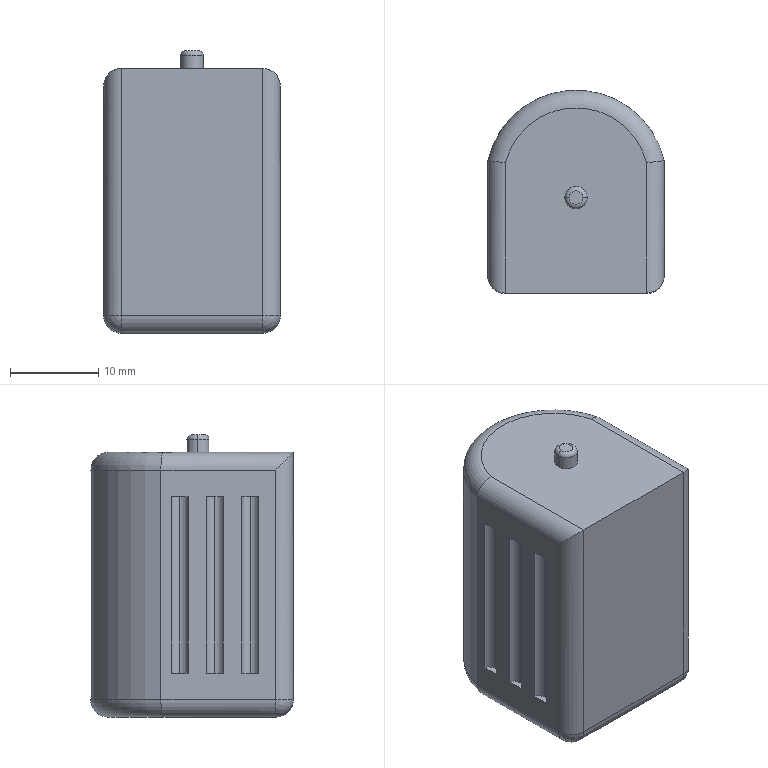Part | SolidWorks | features BaseBody 1 | 1 solid | 43 faces | box 20 x 23 x 32 mm | volume 12308 mm3 | cylinder 19 | plane 18 | torus 4 | sphere 2 | commonest cylinder face diameters 2 x9 4 x7 2.538 x2 20.5 x1
STEP:
#1=CARTESIAN_POINT('',(-1.269,3.315,16.5));
#2=VERTEX_POINT('',#1);
#3=CARTESIAN_POINT('',(1.269,3.315,16.5));
#4=VERTEX_POINT('',#3);
#5=CARTESIAN_POINT('',(0.,3.315,16.5));
#6=DIRECTION('',(0.,0.,-1.));
#7=DIRECTION('',(1.,0.,0.));
#8=AXIS2_PLACEMENT_3D('',#5,#6,#7);
#9=CIRCLE('',#8,1.269);
#10=EDGE_CURVE('',#2,#4,#9,.T.);
#11=ORIENTED_EDGE('',*,*,#10,.F.);
#12=CARTESIAN_POINT('',(-0.7692,3.315,17.));
#13=VERTEX_POINT('',#12);
#14=CARTESIAN_POINT('',(-0.7692,3.315,16.5));
#15=DIRECTION('',(0.,1.,0.));
#16=DIRECTION('',(-1.,0.,0.));
#17=AXIS2_PLACEMENT_3D('',#14,#15,#16);
#18=CIRCLE('',#17,0.5);
#19=EDGE_CURVE('',#2,#13,#18,.T.);
#20=ORIENTED_EDGE('',*,*,#19,.T.);
#21=CARTESIAN_POINT('',(0.7692,3.315,17.));
#22=VERTEX_POINT('',#21);
#23=CARTESIAN_POINT('',(0.,3.315,17.));
#24=DIRECTION('',(0.,0.,1.));
#25=DIRECTION('',(1.,0.,0.));
#26=AXIS2_PLACEMENT_3D('',#23,#24,#25);
#27=CIRCLE('',#26,0.7692);
#28=EDGE_CURVE('',#22,#13,#27,.T.);
#29=ORIENTED_EDGE('',*,*,#28,.F.);
#30=CARTESIAN_POINT('',(0.7692,3.315,16.5));
#31=DIRECTION('',(0.,-1.,0.));
#32=DIRECTION('',(0.,0.,-1.));
#33=AXIS2_PLACEMENT_3D('',#30,#31,#32);
#34=CIRCLE('',#33,0.5);
#35=EDGE_CURVE('',#4,#22,#34,.T.);
#36=ORIENTED_EDGE('',*,*,#35,.F.);
#37=EDGE_LOOP('',(#11,#20,#29,#36));
#38=FACE_OUTER_BOUND('',#37,.T.);
#39=CARTESIAN_POINT('',(0.,3.315,16.5));
#40=DIRECTION('',(0.,0.,1.));
#41=DIRECTION('',(1.,0.,0.));
#42=AXIS2_PLACEMENT_3D('',#39,#40,#41);
#43=TOROIDAL_SURFACE('',#42,0.7692,0.5);
#44=ADVANCED_FACE('',(#38),#43,.T.);
#45=ORIENTED_EDGE('',*,*,#10,.T.);
#46=CARTESIAN_POINT('',(1.269,3.315,15.));
#47=VERTEX_POINT('',#46);
#48=CARTESIAN_POINT('',(1.269,3.315,17.));
#49=DIRECTION('',(0.,0.,-1.));
#50=VECTOR('',#49,1000.);
#51=LINE('',#48,#50);
#52=EDGE_CURVE('',#4,#47,#51,.T.);
#53=ORIENTED_EDGE('',*,*,#52,.T.);
#54=CARTESIAN_POINT('',(-1.269,3.315,15.));
#55=VERTEX_POINT('',#54);
#56=CARTESIAN_POINT('',(0.,3.315,15.));
#57=DIRECTION('',(0.,0.,1.));
#58=DIRECTION('',(-1.,0.,0.));
#59=AXIS2_PLACEMENT_3D('',#56,#57,#58);
#60=CIRCLE('',#59,1.269);
#61=EDGE_CURVE('',#47,#55,#60,.T.);
#62=ORIENTED_EDGE('',*,*,#61,.T.);
#63=CARTESIAN_POINT('',(-1.269,3.315,17.));
#64=DIRECTION('',(0.,0.,-1.));
#65=VECTOR('',#64,1000.);
#66=LINE('',#63,#65);
#67=EDGE_CURVE('',#2,#55,#66,.T.);
#68=ORIENTED_EDGE('',*,*,#67,.F.);
#69=EDGE_LOOP('',(#45,#53,#62,#68));
#70=FACE_OUTER_BOUND('',#69,.T.);
#71=CARTESIAN_POINT('',(0.,3.315,17.));
#72=DIRECTION('',(0.,0.,-1.));
#73=DIRECTION('',(-1.,0.,0.));
#74=AXIS2_PLACEMENT_3D('',#71,#72,#73);
#75=CYLINDRICAL_SURFACE('',#74,1.269);
#76=ADVANCED_FACE('',(#70),#75,.T.);
#77=CARTESIAN_POINT('',(-10.,6.337,-10.));
#78=VERTEX_POINT('',#77);
#79=CARTESIAN_POINT('',(-9.294,5.382,-10.));
#80=VERTEX_POINT('',#79);
#81=CARTESIAN_POINT('',(-10.294,5.382,-10.));
#82=DIRECTION('',(0.,0.,-1.));
#83=DIRECTION('',(-1.,0.,0.));
#84=AXIS2_PLACEMENT_3D('',#81,#82,#83);
#85=CIRCLE('',#84,1.);
#86=EDGE_CURVE('',#78,#80,#85,.T.);
#87=ORIENTED_EDGE('',*,*,#86,.T.);
#88=CARTESIAN_POINT('',(-9.294,5.382,10.));
#89=VERTEX_POINT('',#88);
#90=CARTESIAN_POINT('',(-9.294,5.382,-10.));
#91=DIRECTION('',(0.,0.,1.));
#92=VECTOR('',#91,1000.);
#93=LINE('',#90,#92);
#94=EDGE_CURVE('',#80,#89,#93,.T.);
#95=ORIENTED_EDGE('',*,*,#94,.T.);
#96=CARTESIAN_POINT('',(-10.,6.337,10.));
#97=VERTEX_POINT('',#96);
#98=CARTESIAN_POINT('',(-10.294,5.382,10.));
#99=DIRECTION('',(0.,0.,-1.));
#100=DIRECTION('',(-1.,0.,0.));
#101=AXIS2_PLACEMENT_3D('',#98,#99,#100);
#102=CIRCLE('',#101,1.);
#103=EDGE_CURVE('',#97,#89,#102,.T.);
#104=ORIENTED_EDGE('',*,*,#103,.F.);
#105=CARTESIAN_POINT('',(-10.,6.337,-10.));
#106=DIRECTION('',(0.,0.,-1.));
#107=VECTOR('',#106,1000.);
#108=LINE('',#105,#107);
#109=EDGE_CURVE('',#97,#78,#108,.T.);
#110=ORIENTED_EDGE('',*,*,#109,.T.);
#111=EDGE_LOOP('',(#87,#95,#104,#110));
#112=FACE_OUTER_BOUND('',#111,.T.);
#113=CARTESIAN_POINT('',(-10.294,5.382,-10.));
#114=DIRECTION('',(0.,0.,1.));
#115=DIRECTION('',(1.,0.,0.));
#116=AXIS2_PLACEMENT_3D('',#113,#114,#115);
#117=CYLINDRICAL_SURFACE('',#116,1.);
#118=ADVANCED_FACE('',(#112),#117,.F.);
#119=CARTESIAN_POINT('',(-10.,2.337,-10.));
#120=VERTEX_POINT('',#119);
#121=CARTESIAN_POINT('',(-9.294,1.382,-10.));
#122=VERTEX_POINT('',#121);
#123=CARTESIAN_POINT('',(-10.294,1.382,-10.));
#124=DIRECTION('',(0.,0.,-1.));
#125=DIRECTION('',(-1.,0.,0.));
#126=AXIS2_PLACEMENT_3D('',#123,#124,#125);
#127=CIRCLE('',#126,1.);
#128=EDGE_CURVE('',#120,#122,#127,.T.);
#129=ORIENTED_EDGE('',*,*,#128,.T.);
#130=CARTESIAN_POINT('',(-9.294,1.382,10.));
#131=VERTEX_POINT('',#130);
#132=CARTESIAN_POINT('',(-9.294,1.382,-10.));
#133=DIRECTION('',(0.,0.,1.));
#134=VECTOR('',#133,1000.);
#135=LINE('',#132,#134);
#136=EDGE_CURVE('',#122,#131,#135,.T.);
#137=ORIENTED_EDGE('',*,*,#136,.T.);
#138=CARTESIAN_POINT('',(-10.,2.337,10.));
#139=VERTEX_POINT('',#138);
#140=CARTESIAN_POINT('',(-10.294,1.382,10.));
#141=DIRECTION('',(0.,0.,-1.));
#142=DIRECTION('',(-1.,0.,0.));
#143=AXIS2_PLACEMENT_3D('',#140,#141,#142);
#144=CIRCLE('',#143,1.);
#145=EDGE_CURVE('',#139,#131,#144,.T.);
#146=ORIENTED_EDGE('',*,*,#145,.F.);
#147=CARTESIAN_POINT('',(-10.,2.337,-10.));
#148=DIRECTION('',(0.,0.,-1.));
#149=VECTOR('',#148,1000.);
#150=LINE('',#147,#149);
#151=EDGE_CURVE('',#139,#120,#150,.T.);
#152=ORIENTED_EDGE('',*,*,#151,.T.);
#153=EDGE_LOOP('',(#129,#137,#146,#152));
#154=FACE_OUTER_BOUND('',#153,.T.);
#155=CARTESIAN_POINT('',(-10.294,1.382,-10.));
#156=DIRECTION('',(0.,0.,1.));
#157=DIRECTION('',(1.,0.,0.));
#158=AXIS2_PLACEMENT_3D('',#155,#156,#157);
#159=CYLINDRICAL_SURFACE('',#158,1.);
#160=ADVANCED_FACE('',(#154),#159,.F.);
#161=CARTESIAN_POINT('',(-10.,-1.663,-10.));
#162=VERTEX_POINT('',#161);
#163=CARTESIAN_POINT('',(-9.294,-2.618,-10.));
#164=VERTEX_POINT('',#163);
#165=CARTESIAN_POINT('',(-10.294,-2.618,-10.));
#166=DIRECTION('',(0.,0.,-1.));
#167=DIRECTION('',(-1.,0.,0.));
#168=AXIS2_PLACEMENT_3D('',#165,#166,#167);
#169=CIRCLE('',#168,1.);
#170=EDGE_CURVE('',#162,#164,#169,.T.);
#171=ORIENTED_EDGE('',*,*,#170,.T.);
#172=CARTESIAN_POINT('',(-9.294,-2.618,10.));
#173=VERTEX_POINT('',#172);
#174=CARTESIAN_POINT('',(-9.294,-2.618,-10.));
#175=DIRECTION('',(0.,0.,1.));
#176=VECTOR('',#175,1000.);
#177=LINE('',#174,#176);
#178=EDGE_CURVE('',#164,#173,#177,.T.);
#179=ORIENTED_EDGE('',*,*,#178,.T.);
#180=CARTESIAN_POINT('',(-10.,-1.663,10.));
#181=VERTEX_POINT('',#180);
#182=CARTESIAN_POINT('',(-10.294,-2.618,10.));
#183=DIRECTION('',(0.,0.,-1.));
#184=DIRECTION('',(-1.,0.,0.));
#185=AXIS2_PLACEMENT_3D('',#182,#183,#184);
#186=CIRCLE('',#185,1.);
#187=EDGE_CURVE('',#181,#173,#186,.T.);
#188=ORIENTED_EDGE('',*,*,#187,.F.);
#189=CARTESIAN_POINT('',(-10.,-1.663,-10.));
#190=DIRECTION('',(0.,0.,-1.));
#191=VECTOR('',#190,1000.);
#192=LINE('',#189,#191);
#193=EDGE_CURVE('',#181,#162,#192,.T.);
#194=ORIENTED_EDGE('',*,*,#193,.T.);
#195=EDGE_LOOP('',(#171,#179,#188,#194));
#196=FACE_OUTER_BOUND('',#195,.T.);
#197=CARTESIAN_POINT('',(-10.294,-2.618,-10.));
#198=DIRECTION('',(0.,0.,1.));
#199=DIRECTION('',(1.,0.,0.));
#200=AXIS2_PLACEMENT_3D('',#197,#198,#199);
#201=CYLINDRICAL_SURFACE('',#200,1.);
#202=ADVANCED_FACE('',(#196),#201,.F.);
#203=CARTESIAN_POINT('',(-10.,0.4257,-10.));
#204=VERTEX_POINT('',#203);
#205=CARTESIAN_POINT('',(-10.,7.5,-10.));
#206=DIRECTION('',(0.,-1.,0.));
#207=VECTOR('',#206,1000.);
#208=LINE('',#205,#207);
#209=EDGE_CURVE('',#120,#204,#208,.T.);
#210=ORIENTED_EDGE('',*,*,#209,.F.);
#211=ORIENTED_EDGE('',*,*,#151,.F.);
#212=CARTESIAN_POINT('',(-10.,0.4257,10.));
#213=VERTEX_POINT('',#212);
#214=CARTESIAN_POINT('',(-10.,7.5,10.));
#215=DIRECTION('',(0.,-1.,0.));
#216=VECTOR('',#215,1000.);
#217=LINE('',#214,#216);
#218=EDGE_CURVE('',#139,#213,#217,.T.);
#219=ORIENTED_EDGE('',*,*,#218,.T.);
#220=CARTESIAN_POINT('',(-10.,0.4257,-10.));
#221=DIRECTION('',(0.,0.,1.));
#222=VECTOR('',#221,1000.);
#223=LINE('',#220,#222);
#224=EDGE_CURVE('',#204,#213,#223,.T.);
#225=ORIENTED_EDGE('',*,*,#224,.F.);
#226=EDGE_LOOP('',(#210,#211,#219,#225));
#227=FACE_BOUND('',#226,.T.);
#228=CARTESIAN_POINT('',(-10.,7.5,13.));
#229=VERTEX_POINT('',#228);
#230=CARTESIAN_POINT('',(-10.,7.5,-13.));
#231=VERTEX_POINT('',#230);
#232=CARTESIAN_POINT('',(-10.,7.5,15.));
#233=DIRECTION('',(0.,0.,-1.));
#234=VECTOR('',#233,1000.);
#235=LINE('',#232,#234);
#236=EDGE_CURVE('',#229,#231,#235,.T.);
#237=ORIENTED_EDGE('',*,*,#236,.T.);
#238=CARTESIAN_POINT('',(-10.,-5.5,-13.));
#239=VERTEX_POINT('',#238);
#240=CARTESIAN_POINT('',(-10.,-7.5,-13.));
#241=DIRECTION('',(0.,-1.,0.));
#242=VECTOR('',#241,1000.);
#243=LINE('',#240,#242);
#244=EDGE_CURVE('',#231,#239,#243,.T.);
#245=ORIENTED_EDGE('',*,*,#244,.T.);
#246=CARTESIAN_POINT('',(-10.,-5.5,13.));
#247=VERTEX_POINT('',#246);
#248=CARTESIAN_POINT('',(-10.,-5.5,15.));
#249=DIRECTION('',(0.,0.,1.));
#250=VECTOR('',#249,1000.);
#251=LINE('',#248,#250);
#252=EDGE_CURVE('',#239,#247,#251,.T.);
#253=ORIENTED_EDGE('',*,*,#252,.T.);
#254=CARTESIAN_POINT('',(-10.,7.5,13.));
#255=DIRECTION('',(0.,1.,0.));
#256=VECTOR('',#255,1000.);
#257=LINE('',#254,#256);
#258=EDGE_CURVE('',#247,#229,#257,.T.);
#259=ORIENTED_EDGE('',*,*,#258,.T.);
#260=EDGE_LOOP('',(#237,#245,#253,#259));
#261=FACE_OUTER_BOUND('',#260,.T.);
#262=CARTESIAN_POINT('',(-10.,-3.574,-10.));
#263=VERTEX_POINT('',#262);
#264=CARTESIAN_POINT('',(-10.,7.5,-10.));
#265=DIRECTION('',(0.,-1.,0.));
#266=VECTOR('',#265,1000.);
#267=LINE('',#264,#266);
#268=EDGE_CURVE('',#162,#263,#267,.T.);
#269=ORIENTED_EDGE('',*,*,#268,.F.);
#270=ORIENTED_EDGE('',*,*,#193,.F.);
#271=CARTESIAN_POINT('',(-10.,-3.574,10.));
#272=VERTEX_POINT('',#271);
#273=CARTESIAN_POINT('',(-10.,7.5,10.));
#274=DIRECTION('',(0.,-1.,0.));
#275=VECTOR('',#274,1000.);
#276=LINE('',#273,#275);
#277=EDGE_CURVE('',#181,#272,#276,.T.);
#278=ORIENTED_EDGE('',*,*,#277,.T.);
#279=CARTESIAN_POINT('',(-10.,-3.574,-10.));
#280=DIRECTION('',(0.,0.,1.));
#281=VECTOR('',#280,1000.);
#282=LINE('',#279,#281);
#283=EDGE_CURVE('',#263,#272,#282,.T.);
#284=ORIENTED_EDGE('',*,*,#283,.F.);
#285=EDGE_LOOP('',(#269,#270,#278,#284));
#286=FACE_BOUND('',#285,.T.);
#287=CARTESIAN_POINT('',(-10.,4.426,-10.));
#288=VERTEX_POINT('',#287);
#289=CARTESIAN_POINT('',(-10.,7.5,-10.));
#290=DIRECTION('',(0.,-1.,0.));
#291=VECTOR('',#290,1000.);
#292=LINE('',#289,#291);
#293=EDGE_CURVE('',#78,#288,#292,.T.);
#294=ORIENTED_EDGE('',*,*,#293,.F.);
#295=ORIENTED_EDGE('',*,*,#109,.F.);
#296=CARTESIAN_POINT('',(-10.,4.426,10.));
#297=VERTEX_POINT('',#296);
#298=CARTESIAN_POINT('',(-10.,7.5,10.));
#299=DIRECTION('',(0.,-1.,0.));
#300=VECTOR('',#299,1000.);
#301=LINE('',#298,#300);
#302=EDGE_CURVE('',#97,#297,#301,.T.);
#303=ORIENTED_EDGE('',*,*,#302,.T.);
#304=CARTESIAN_POINT('',(-10.,4.426,-10.));
#305=DIRECTION('',(0.,0.,1.));
#306=VECTOR('',#305,1000.);
#307=LINE('',#304,#306);
#308=EDGE_CURVE('',#288,#297,#307,.T.);
#309=ORIENTED_EDGE('',*,*,#308,.F.);
#310=EDGE_LOOP('',(#294,#295,#303,#309));
#311=FACE_BOUND('',#310,.T.);
#312=CARTESIAN_POINT('',(-10.,7.5,15.));
#313=DIRECTION('',(1.,0.,0.));
#314=DIRECTION('',(0.,0.,-1.));
#315=AXIS2_PLACEMENT_3D('',#312,#313,#314);
#316=PLANE('',#315);
#317=ADVANCED_FACE('',(#227,#261,#286,#311),#316,.F.);
#318=CARTESIAN_POINT('',(10.,-3.574,-10.));
#319=VERTEX_POINT('',#318);
#320=CARTESIAN_POINT('',(10.,-1.663,-10.));
#321=VERTEX_POINT('',#320);
#322=CARTESIAN_POINT('',(10.,7.5,-10.));
#323=DIRECTION('',(0.,1.,0.));
#324=VECTOR('',#323,1000.);
#325=LINE('',#322,#324);
#326=EDGE_CURVE('',#319,#321,#325,.T.);
#327=ORIENTED_EDGE('',*,*,#326,.F.);
#328=CARTESIAN_POINT('',(10.,-3.574,10.));
#329=VERTEX_POINT('',#328);
#330=CARTESIAN_POINT('',(10.,-3.574,-10.));
#331=DIRECTION('',(0.,0.,1.));
#332=VECTOR('',#331,1000.);
#333=LINE('',#330,#332);
#334=EDGE_CURVE('',#319,#329,#333,.T.);
#335=ORIENTED_EDGE('',*,*,#334,.T.);
#336=CARTESIAN_POINT('',(10.,-1.663,10.));
#337=VERTEX_POINT('',#336);
#338=CARTESIAN_POINT('',(10.,7.5,10.));
#339=DIRECTION('',(0.,1.,0.));
#340=VECTOR('',#339,1000.);
#341=LINE('',#338,#340);
#342=EDGE_CURVE('',#329,#337,#341,.T.);
#343=ORIENTED_EDGE('',*,*,#342,.T.);
#344=CARTESIAN_POINT('',(10.,-1.663,-10.));
#345=DIRECTION('',(0.,0.,-1.));
#346=VECTOR('',#345,1000.);
#347=LINE('',#344,#346);
#348=EDGE_CURVE('',#337,#321,#347,.T.);
#349=ORIENTED_EDGE('',*,*,#348,.T.);
#350=EDGE_LOOP('',(#327,#335,#343,#349));
#351=FACE_BOUND('',#350,.T.);
#352=CARTESIAN_POINT('',(10.,-5.5,13.));
#353=VERTEX_POINT('',#352);
#354=CARTESIAN_POINT('',(10.,-5.5,-13.));
#355=VERTEX_POINT('',#354);
#356=CARTESIAN_POINT('',(10.,-5.5,15.));
#357=DIRECTION('',(0.,0.,-1.));
#358=VECTOR('',#357,1000.);
#359=LINE('',#356,#358);
#360=EDGE_CURVE('',#353,#355,#359,.T.);
#361=ORIENTED_EDGE('',*,*,#360,.T.);
#362=CARTESIAN_POINT('',(10.,7.5,-13.));
#363=VERTEX_POINT('',#362);
#364=CARTESIAN_POINT('',(10.,7.5,-13.));
#365=DIRECTION('',(0.,1.,0.));
#366=VECTOR('',#365,1000.);
#367=LINE('',#364,#366);
#368=EDGE_CURVE('',#355,#363,#367,.T.);
#369=ORIENTED_EDGE('',*,*,#368,.T.);
#370=CARTESIAN_POINT('',(10.,7.5,13.));
#371=VERTEX_POINT('',#370);
#372=CARTESIAN_POINT('',(10.,7.5,15.));
#373=DIRECTION('',(0.,0.,-1.));
#374=VECTOR('',#373,1000.);
#375=LINE('',#372,#374);
#376=EDGE_CURVE('',#371,#363,#375,.T.);
#377=ORIENTED_EDGE('',*,*,#376,.F.);
#378=CARTESIAN_POINT('',(10.,7.5,13.));
#379=DIRECTION('',(0.,-1.,0.));
#380=VECTOR('',#379,1000.);
#381=LINE('',#378,#380);
#382=EDGE_CURVE('',#371,#353,#381,.T.);
#383=ORIENTED_EDGE('',*,*,#382,.T.);
#384=EDGE_LOOP('',(#361,#369,#377,#383));
#385=FACE_OUTER_BOUND('',#384,.T.);
#386=CARTESIAN_POINT('',(10.,4.426,-10.));
#387=VERTEX_POINT('',#386);
#388=CARTESIAN_POINT('',(10.,6.337,-10.));
#389=VERTEX_POINT('',#388);
#390=CARTESIAN_POINT('',(10.,7.5,-10.));
#391=DIRECTION('',(0.,1.,0.));
#392=VECTOR('',#391,1000.);
#393=LINE('',#390,#392);
#394=EDGE_CURVE('',#387,#389,#393,.T.);
#395=ORIENTED_EDGE('',*,*,#394,.F.);
#396=CARTESIAN_POINT('',(10.,4.426,10.));
#397=VERTEX_POINT('',#396);
#398=CARTESIAN_POINT('',(10.,4.426,-10.));
#399=DIRECTION('',(0.,0.,1.));
#400=VECTOR('',#399,1000.);
#401=LINE('',#398,#400);
#402=EDGE_CURVE('',#387,#397,#401,.T.);
#403=ORIENTED_EDGE('',*,*,#402,.T.);
#404=CARTESIAN_POINT('',(10.,6.337,10.));
#405=VERTEX_POINT('',#404);
#406=CARTESIAN_POINT('',(10.,7.5,10.));
#407=DIRECTION('',(0.,1.,0.));
#408=VECTOR('',#407,1000.);
#409=LINE('',#406,#408);
#410=EDGE_CURVE('',#397,#405,#409,.T.);
#411=ORIENTED_EDGE('',*,*,#410,.T.);
#412=CARTESIAN_POINT('',(10.,6.337,-10.));
#413=DIRECTION('',(0.,0.,-1.));
#414=VECTOR('',#413,1000.);
#415=LINE('',#412,#414);
#416=EDGE_CURVE('',#405,#389,#415,.T.);
#417=ORIENTED_EDGE('',*,*,#416,.T.);
#418=EDGE_LOOP('',(#395,#403,#411,#417));
#419=FACE_BOUND('',#418,.T.);
#420=CARTESIAN_POINT('',(10.,0.4257,-10.));
#421=VERTEX_POINT('',#420);
#422=CARTESIAN_POINT('',(10.,2.337,-10.));
#423=VERTEX_POINT('',#422);
#424=CARTESIAN_POINT('',(10.,7.5,-10.));
#425=DIRECTION('',(0.,1.,0.));
#426=VECTOR('',#425,1000.);
#427=LINE('',#424,#426);
#428=EDGE_CURVE('',#421,#423,#427,.T.);
#429=ORIENTED_EDGE('',*,*,#428,.F.);
#430=CARTESIAN_POINT('',(10.,0.4257,10.));
#431=VERTEX_POINT('',#430);
#432=CARTESIAN_POINT('',(10.,0.4257,-10.));
#433=DIRECTION('',(0.,0.,1.));
#434=VECTOR('',#433,1000.);
#435=LINE('',#432,#434);
#436=EDGE_CURVE('',#421,#431,#435,.T.);
#437=ORIENTED_EDGE('',*,*,#436,.T.);
#438=CARTESIAN_POINT('',(10.,2.337,10.));
#439=VERTEX_POINT('',#438);
#440=CARTESIAN_POINT('',(10.,7.5,10.));
#441=DIRECTION('',(0.,1.,0.));
#442=VECTOR('',#441,1000.);
#443=LINE('',#440,#442);
#444=EDGE_CURVE('',#431,#439,#443,.T.);
#445=ORIENTED_EDGE('',*,*,#444,.T.);
#446=CARTESIAN_POINT('',(10.,2.337,-10.));
#447=DIRECTION('',(0.,0.,-1.));
#448=VECTOR('',#447,1000.);
#449=LINE('',#446,#448);
#450=EDGE_CURVE('',#439,#423,#449,.T.);
#451=ORIENTED_EDGE('',*,*,#450,.T.);
#452=EDGE_LOOP('',(#429,#437,#445,#451));
#453=FACE_BOUND('',#452,.T.);
#454=CARTESIAN_POINT('',(10.,7.5,15.));
#455=DIRECTION('',(-1.,0.,0.));
#456=DIRECTION('',(0.,0.,1.));
#457=AXIS2_PLACEMENT_3D('',#454,#455,#456);
#458=PLANE('',#457);
#459=ADVANCED_FACE('',(#351,#385,#419,#453),#458,.F.);
#460=ORIENTED_EDGE('',*,*,#376,.T.);
#461=CARTESIAN_POINT('',(0.,5.25,-13.));
#462=DIRECTION('',(0.,0.,1.));
#463=DIRECTION('',(-1.,0.,0.));
#464=AXIS2_PLACEMENT_3D('',#461,#462,#463);
#465=CIRCLE('',#464,10.25);
#466=EDGE_CURVE('',#363,#231,#465,.T.);
#467=ORIENTED_EDGE('',*,*,#466,.T.);
#468=ORIENTED_EDGE('',*,*,#236,.F.);
#469=CARTESIAN_POINT('',(0.,5.25,13.));
#470=DIRECTION('',(0.,0.,-1.));
#471=DIRECTION('',(-1.,0.,0.));
#472=AXIS2_PLACEMENT_3D('',#469,#470,#471);
#473=CIRCLE('',#472,10.25);
#474=EDGE_CURVE('',#229,#371,#473,.T.);
#475=ORIENTED_EDGE('',*,*,#474,.T.);
#476=EDGE_LOOP('',(#460,#467,#468,#475));
#477=FACE_OUTER_BOUND('',#476,.T.);
#478=CARTESIAN_POINT('',(0.,5.25,15.));
#479=DIRECTION('',(0.,0.,-1.));
#480=DIRECTION('',(-1.,0.,0.));
#481=AXIS2_PLACEMENT_3D('',#478,#479,#480);
#482=CYLINDRICAL_SURFACE('',#481,10.25);
#483=ADVANCED_FACE('',(#477),#482,.T.);
#484=CARTESIAN_POINT('',(-8.,-7.5,15.));
#485=VERTEX_POINT('',#484);
#486=CARTESIAN_POINT('',(8.,-7.5,15.));
#487=VERTEX_POINT('',#486);
#488=CARTESIAN_POINT('',(-10.,-7.5,15.));
#489=DIRECTION('',(1.,0.,0.));
#490=VECTOR('',#489,1000.);
#491=LINE('',#488,#490);
#492=EDGE_CURVE('',#485,#487,#491,.T.);
#493=ORIENTED_EDGE('',*,*,#492,.F.);
#494=CARTESIAN_POINT('',(-8.,-7.5,-13.));
#495=VERTEX_POINT('',#494);
#496=CARTESIAN_POINT('',(-8.,-7.5,15.));
#497=DIRECTION('',(0.,0.,-1.));
#498=VECTOR('',#497,1000.);
#499=LINE('',#496,#498);
#500=EDGE_CURVE('',#485,#495,#499,.T.);
#501=ORIENTED_EDGE('',*,*,#500,.T.);
#502=CARTESIAN_POINT('',(8.,-7.5,-13.));
#503=VERTEX_POINT('',#502);
#504=CARTESIAN_POINT('',(10.,-7.5,-13.));
#505=DIRECTION('',(1.,0.,0.));
#506=VECTOR('',#505,1000.);
#507=LINE('',#504,#506);
#508=EDGE_CURVE('',#495,#503,#507,.T.);
#509=ORIENTED_EDGE('',*,*,#508,.T.);
#510=CARTESIAN_POINT('',(8.,-7.5,15.));
#511=DIRECTION('',(0.,0.,1.));
#512=VECTOR('',#511,1000.);
#513=LINE('',#510,#512);
#514=EDGE_CURVE('',#503,#487,#513,.T.);
#515=ORIENTED_EDGE('',*,*,#514,.T.);
#516=EDGE_LOOP('',(#493,#501,#509,#515));
#517=FACE_OUTER_BOUND('',#516,.T.);
#518=CARTESIAN_POINT('',(-10.,-7.5,15.));
#519=DIRECTION('',(0.,1.,0.));
#520=DIRECTION('',(0.,0.,1.));
#521=AXIS2_PLACEMENT_3D('',#518,#519,#520);
#522=PLANE('',#521);
#523=ADVANCED_FACE('',(#517),#522,.F.);
#524=CARTESIAN_POINT('',(0.,3.315,15.));
#525=DIRECTION('',(0.,0.,1.));
#526=DIRECTION('',(-1.,0.,0.));
#527=AXIS2_PLACEMENT_3D('',#524,#525,#526);
#528=CIRCLE('',#527,1.269);
#529=EDGE_CURVE('',#55,#47,#528,.T.);
#530=ORIENTED_EDGE('',*,*,#529,.F.);
#531=ORIENTED_EDGE('',*,*,#61,.F.);
#532=EDGE_LOOP('',(#530,#531));
#533=FACE_BOUND('',#532,.T.);
#534=ORIENTED_EDGE('',*,*,#492,.T.);
#535=CARTESIAN_POINT('',(8.,7.266,15.));
#536=VERTEX_POINT('',#535);
#537=CARTESIAN_POINT('',(8.,5.25,15.));
#538=DIRECTION('',(0.,1.,0.));
#539=VECTOR('',#538,1000.);
#540=LINE('',#537,#539);
#541=EDGE_CURVE('',#487,#536,#540,.T.);
#542=ORIENTED_EDGE('',*,*,#541,.T.);
#543=CARTESIAN_POINT('',(-8.,7.266,15.));
#544=VERTEX_POINT('',#543);
#545=CARTESIAN_POINT('',(0.,5.25,15.));
#546=DIRECTION('',(0.,0.,1.));
#547=DIRECTION('',(-1.,0.,0.));
#548=AXIS2_PLACEMENT_3D('',#545,#546,#547);
#549=CIRCLE('',#548,8.25);
#550=EDGE_CURVE('',#536,#544,#549,.T.);
#551=ORIENTED_EDGE('',*,*,#550,.T.);
#552=CARTESIAN_POINT('',(-8.,5.25,15.));
#553=DIRECTION('',(0.,-1.,0.));
#554=VECTOR('',#553,1000.);
#555=LINE('',#552,#554);
#556=EDGE_CURVE('',#544,#485,#555,.T.);
#557=ORIENTED_EDGE('',*,*,#556,.T.);
#558=EDGE_LOOP('',(#534,#542,#551,#557));
#559=FACE_OUTER_BOUND('',#558,.T.);
#560=CARTESIAN_POINT('',(0.,5.25,15.));
#561=DIRECTION('',(0.,0.,-1.));
#562=DIRECTION('',(-1.,0.,0.));
#563=AXIS2_PLACEMENT_3D('',#560,#561,#562);
#564=PLANE('',#563);
#565=ADVANCED_FACE('',(#533,#559),#564,.F.);
#566=CARTESIAN_POINT('',(8.,-5.5,-15.));
#567=VERTEX_POINT('',#566);
#568=CARTESIAN_POINT('',(-8.,-5.5,-15.));
#569=VERTEX_POINT('',#568);
#570=CARTESIAN_POINT('',(-10.,-5.5,-15.));
#571=DIRECTION('',(-1.,0.,0.));
#572=VECTOR('',#571,1000.);
#573=LINE('',#570,#572);
#574=EDGE_CURVE('',#567,#569,#573,.T.);
#575=ORIENTED_EDGE('',*,*,#574,.T.);
#576=CARTESIAN_POINT('',(-8.,7.266,-15.));
#577=VERTEX_POINT('',#576);
#578=CARTESIAN_POINT('',(-8.,7.5,-15.));
#579=DIRECTION('',(0.,1.,0.));
#580=VECTOR('',#579,1000.);
#581=LINE('',#578,#580);
#582=EDGE_CURVE('',#569,#577,#581,.T.);
#583=ORIENTED_EDGE('',*,*,#582,.T.);
#584=CARTESIAN_POINT('',(8.,7.266,-15.));
#585=VERTEX_POINT('',#584);
#586=CARTESIAN_POINT('',(0.,5.25,-15.));
#587=DIRECTION('',(0.,0.,-1.));
#588=DIRECTION('',(-1.,0.,0.));
#589=AXIS2_PLACEMENT_3D('',#586,#587,#588);
#590=CIRCLE('',#589,8.25);
#591=EDGE_CURVE('',#577,#585,#590,.T.);
#592=ORIENTED_EDGE('',*,*,#591,.T.);
#593=CARTESIAN_POINT('',(8.,-7.5,-15.));
#594=DIRECTION('',(0.,-1.,0.));
#595=VECTOR('',#594,1000.);
#596=LINE('',#593,#595);
#597=EDGE_CURVE('',#585,#567,#596,.T.);
#598=ORIENTED_EDGE('',*,*,#597,.T.);
#599=EDGE_LOOP('',(#575,#583,#592,#598));
#600=FACE_OUTER_BOUND('',#599,.T.);
#601=CARTESIAN_POINT('',(0.,5.25,-15.));
#602=DIRECTION('',(0.,0.,-1.));
#603=DIRECTION('',(-1.,0.,0.));
#604=AXIS2_PLACEMENT_3D('',#601,#602,#603);
#605=PLANE('',#604);
#606=ADVANCED_FACE('',(#600),#605,.T.);
#607=CARTESIAN_POINT('',(10.,-5.5,13.));
#608=CARTESIAN_POINT('',(10.,-6.672,14.172));
#609=CARTESIAN_POINT('',(9.172,-7.5,15.));
#610=CARTESIAN_POINT('',(8.,-7.5,15.));
#611=(BOUNDED_CURVE()B_SPLINE_CURVE(3,(#607,#608,#609,#610),.UNSPECIFIED.,.F.,.T.)B_SPLINE_CURVE_WITH_KNOTS((4,4),(1.571,3.142),.UNSPECIFIED.)CURVE()GEOMETRIC_REPRESENTATION_ITEM()RATIONAL_B_SPLINE_CURVE((1.,0.8047,0.8047,1.))REPRESENTATION_ITEM(''));
#612=EDGE_CURVE('',#353,#487,#611,.T.);
#613=ORIENTED_EDGE('',*,*,#612,.F.);
#614=ORIENTED_EDGE('',*,*,#382,.F.);
#615=CARTESIAN_POINT('',(8.,7.266,15.));
#616=CARTESIAN_POINT('',(8.261,7.298,15.));
#617=CARTESIAN_POINT('',(8.525,7.33,14.947));
#618=CARTESIAN_POINT('',(9.005,7.387,14.749));
#619=CARTESIAN_POINT('',(9.228,7.413,14.6));
#620=CARTESIAN_POINT('',(9.505,7.444,14.324));
#621=CARTESIAN_POINT('',(9.589,7.454,14.221));
#622=CARTESIAN_POINT('',(9.735,7.47,14.004));
#623=CARTESIAN_POINT('',(9.796,7.477,13.889));
#624=CARTESIAN_POINT('',(9.897,7.489,13.646));
#625=CARTESIAN_POINT('',(9.936,7.493,13.519));
#626=CARTESIAN_POINT('',(9.987,7.499,13.263));
#627=CARTESIAN_POINT('',(10.,7.5,13.133));
#628=CARTESIAN_POINT('',(10.,7.5,13.));
#629=B_SPLINE_CURVE_WITH_KNOTS('',3,(#615,#616,#617,#618,#619,#620,#621,#622,#623,#624,#625,#626,#627,#628),.UNSPECIFIED.,.F.,.F.,(4,2,2,2,2,2,4),(-0.0000181,0.0007721,0.001562,0.001958,0.002353,0.002748,0.003143),.UNSPECIFIED.);
#630=EDGE_CURVE('',#536,#371,#629,.T.);
#631=ORIENTED_EDGE('',*,*,#630,.F.);
#632=ORIENTED_EDGE('',*,*,#541,.F.);
#633=EDGE_LOOP('',(#613,#614,#631,#632));
#634=FACE_OUTER_BOUND('',#633,.T.);
#635=CARTESIAN_POINT('',(8.,5.25,13.));
#636=DIRECTION('',(0.,1.,0.));
#637=DIRECTION('',(0.,0.,1.));
#638=AXIS2_PLACEMENT_3D('',#635,#636,#637);
#639=CYLINDRICAL_SURFACE('',#638,2.);
#640=ADVANCED_FACE('',(#634),#639,.T.);
#641=ORIENTED_EDGE('',*,*,#630,.T.);
#642=ORIENTED_EDGE('',*,*,#474,.F.);
#643=CARTESIAN_POINT('',(-8.,7.266,15.));
#644=CARTESIAN_POINT('',(-8.261,7.298,15.));
#645=CARTESIAN_POINT('',(-8.525,7.33,14.947));
#646=CARTESIAN_POINT('',(-9.005,7.387,14.749));
#647=CARTESIAN_POINT('',(-9.228,7.413,14.6));
#648=CARTESIAN_POINT('',(-9.505,7.444,14.324));
#649=CARTESIAN_POINT('',(-9.589,7.454,14.221));
#650=CARTESIAN_POINT('',(-9.735,7.47,14.004));
#651=CARTESIAN_POINT('',(-9.796,7.477,13.889));
#652=CARTESIAN_POINT('',(-9.897,7.489,13.646));
#653=CARTESIAN_POINT('',(-9.936,7.493,13.519));
#654=CARTESIAN_POINT('',(-9.987,7.499,13.263));
#655=CARTESIAN_POINT('',(-10.,7.5,13.133));
#656=CARTESIAN_POINT('',(-10.,7.5,13.));
#657=B_SPLINE_CURVE_WITH_KNOTS('',3,(#643,#644,#645,#646,#647,#648,#649,#650,#651,#652,#653,#654,#655,#656),.UNSPECIFIED.,.F.,.F.,(4,2,2,2,2,2,4),(-0.0000181,0.0007721,0.001562,0.001958,0.002353,0.002748,0.003143),.UNSPECIFIED.);
#658=EDGE_CURVE('',#544,#229,#657,.T.);
#659=ORIENTED_EDGE('',*,*,#658,.F.);
#660=ORIENTED_EDGE('',*,*,#550,.F.);
#661=EDGE_LOOP('',(#641,#642,#659,#660));
#662=FACE_OUTER_BOUND('',#661,.T.);
#663=CARTESIAN_POINT('',(0.,5.25,13.));
#664=DIRECTION('',(0.,0.,-1.));
#665=DIRECTION('',(-1.,0.,0.));
#666=AXIS2_PLACEMENT_3D('',#663,#664,#665);
#667=TOROIDAL_SURFACE('',#666,8.25,2.);
#668=ADVANCED_FACE('',(#662),#667,.T.);
#669=ORIENTED_EDGE('',*,*,#612,.T.);
#670=ORIENTED_EDGE('',*,*,#514,.F.);
#671=CARTESIAN_POINT('',(8.,-5.5,-13.));
#672=DIRECTION('',(0.,0.,-1.));
#673=DIRECTION('',(-1.,0.,0.));
#674=AXIS2_PLACEMENT_3D('',#671,#672,#673);
#675=CIRCLE('',#674,2.);
#676=EDGE_CURVE('',#355,#503,#675,.T.);
#677=ORIENTED_EDGE('',*,*,#676,.F.);
#678=ORIENTED_EDGE('',*,*,#360,.F.);
#679=EDGE_LOOP('',(#669,#670,#677,#678));
#680=FACE_OUTER_BOUND('',#679,.T.);
#681=CARTESIAN_POINT('',(8.,-5.5,15.));
#682=DIRECTION('',(0.,0.,-1.));
#683=DIRECTION('',(-1.,0.,0.));
#684=AXIS2_PLACEMENT_3D('',#681,#682,#683);
#685=CYLINDRICAL_SURFACE('',#684,2.);
#686=ADVANCED_FACE('',(#680),#685,.T.);
#687=ORIENTED_EDGE('',*,*,#658,.T.);
#688=ORIENTED_EDGE('',*,*,#258,.F.);
#689=CARTESIAN_POINT('',(-8.,-7.5,15.));
#690=CARTESIAN_POINT('',(-9.172,-7.5,15.));
#691=CARTESIAN_POINT('',(-10.,-6.672,14.172));
#692=CARTESIAN_POINT('',(-10.,-5.5,13.));
#693=(BOUNDED_CURVE()B_SPLINE_CURVE(3,(#689,#690,#691,#692),.UNSPECIFIED.,.F.,.F.)B_SPLINE_CURVE_WITH_KNOTS((4,4),(3.142,4.712),.UNSPECIFIED.)CURVE()GEOMETRIC_REPRESENTATION_ITEM()RATIONAL_B_SPLINE_CURVE((1.,0.8047,0.8047,1.))REPRESENTATION_ITEM(''));
#694=EDGE_CURVE('',#485,#247,#693,.T.);
#695=ORIENTED_EDGE('',*,*,#694,.F.);
#696=ORIENTED_EDGE('',*,*,#556,.F.);
#697=EDGE_LOOP('',(#687,#688,#695,#696));
#698=FACE_OUTER_BOUND('',#697,.T.);
#699=CARTESIAN_POINT('',(-8.,5.25,13.));
#700=DIRECTION('',(0.,-1.,0.));
#701=DIRECTION('',(0.,0.,-1.));
#702=AXIS2_PLACEMENT_3D('',#699,#700,#701);
#703=CYLINDRICAL_SURFACE('',#702,2.);
#704=ADVANCED_FACE('',(#698),#703,.T.);
#705=CARTESIAN_POINT('',(8.,-5.5,-13.));
#706=DIRECTION('',(-1.,0.,0.));
#707=DIRECTION('',(0.,0.,-1.));
#708=AXIS2_PLACEMENT_3D('',#705,#706,#707);
#709=CIRCLE('',#708,2.);
#710=EDGE_CURVE('',#567,#503,#709,.T.);
#711=ORIENTED_EDGE('',*,*,#710,.F.);
#712=CARTESIAN_POINT('',(8.,-5.5,-13.));
#713=DIRECTION('',(0.,1.,0.));
#714=DIRECTION('',(0.,0.,-1.));
#715=AXIS2_PLACEMENT_3D('',#712,#713,#714);
#716=CIRCLE('',#715,2.);
#717=EDGE_CURVE('',#355,#567,#716,.T.);
#718=ORIENTED_EDGE('',*,*,#717,.F.);
#719=ORIENTED_EDGE('',*,*,#676,.T.);
#720=EDGE_LOOP('',(#711,#718,#719));
#721=FACE_OUTER_BOUND('',#720,.T.);
#722=CARTESIAN_POINT('',(8.,-5.5,-13.));
#723=DIRECTION('',(0.,1.,0.));
#724=DIRECTION('',(1.,0.,0.));
#725=AXIS2_PLACEMENT_3D('',#722,#723,#724);
#726=SPHERICAL_SURFACE('',#725,2.);
#727=ADVANCED_FACE('',(#721),#726,.T.);
#728=ORIENTED_EDGE('',*,*,#717,.T.);
#729=ORIENTED_EDGE('',*,*,#597,.F.);
#730=CARTESIAN_POINT('',(10.,7.5,-13.));
#731=CARTESIAN_POINT('',(10.,7.5,-13.133));
#732=CARTESIAN_POINT('',(9.987,7.499,-13.263));
#733=CARTESIAN_POINT('',(9.936,7.493,-13.519));
#734=CARTESIAN_POINT('',(9.897,7.489,-13.646));
#735=CARTESIAN_POINT('',(9.796,7.477,-13.889));
#736=CARTESIAN_POINT('',(9.735,7.47,-14.004));
#737=CARTESIAN_POINT('',(9.589,7.454,-14.221));
#738=CARTESIAN_POINT('',(9.504,7.444,-14.324));
#739=CARTESIAN_POINT('',(9.227,7.413,-14.6));
#740=CARTESIAN_POINT('',(9.004,7.387,-14.749));
#741=CARTESIAN_POINT('',(8.524,7.33,-14.947));
#742=CARTESIAN_POINT('',(8.259,7.298,-15.));
#743=CARTESIAN_POINT('',(8.,7.266,-15.));
#744=B_SPLINE_CURVE_WITH_KNOTS('',3,(#730,#731,#732,#733,#734,#735,#736,#737,#738,#739,#740,#741,#742,#743),.UNSPECIFIED.,.F.,.F.,(4,2,2,2,2,2,4),(0.,0.0003919,0.0007838,0.001176,0.001568,0.002351,0.003135),.UNSPECIFIED.);
#745=EDGE_CURVE('',#363,#585,#744,.T.);
#746=ORIENTED_EDGE('',*,*,#745,.F.);
#747=ORIENTED_EDGE('',*,*,#368,.F.);
#748=EDGE_LOOP('',(#728,#729,#746,#747));
#749=FACE_OUTER_BOUND('',#748,.T.);
#750=CARTESIAN_POINT('',(8.,7.5,-13.));
#751=DIRECTION('',(0.,-1.,0.));
#752=DIRECTION('',(0.,0.,-1.));
#753=AXIS2_PLACEMENT_3D('',#750,#751,#752);
#754=CYLINDRICAL_SURFACE('',#753,2.);
#755=ADVANCED_FACE('',(#749),#754,.T.);
#756=ORIENTED_EDGE('',*,*,#694,.T.);
#757=ORIENTED_EDGE('',*,*,#252,.F.);
#758=CARTESIAN_POINT('',(-8.,-5.5,-13.));
#759=DIRECTION('',(0.,0.,-1.));
#760=DIRECTION('',(-1.,0.,0.));
#761=AXIS2_PLACEMENT_3D('',#758,#759,#760);
#762=CIRCLE('',#761,2.);
#763=EDGE_CURVE('',#495,#239,#762,.T.);
#764=ORIENTED_EDGE('',*,*,#763,.F.);
#765=ORIENTED_EDGE('',*,*,#500,.F.);
#766=EDGE_LOOP('',(#756,#757,#764,#765));
#767=FACE_OUTER_BOUND('',#766,.T.);
#768=CARTESIAN_POINT('',(-8.,-5.5,15.));
#769=DIRECTION('',(0.,0.,-1.));
#770=DIRECTION('',(-1.,0.,0.));
#771=AXIS2_PLACEMENT_3D('',#768,#769,#770);
#772=CYLINDRICAL_SURFACE('',#771,2.);
#773=ADVANCED_FACE('',(#767),#772,.T.);
#774=ORIENTED_EDGE('',*,*,#710,.T.);
#775=ORIENTED_EDGE('',*,*,#508,.F.);
#776=CARTESIAN_POINT('',(-8.,-5.5,-13.));
#777=DIRECTION('',(-1.,0.,0.));
#778=DIRECTION('',(0.,0.,1.));
#779=AXIS2_PLACEMENT_3D('',#776,#777,#778);
#780=CIRCLE('',#779,2.);
#781=EDGE_CURVE('',#569,#495,#780,.T.);
#782=ORIENTED_EDGE('',*,*,#781,.F.);
#783=ORIENTED_EDGE('',*,*,#574,.F.);
#784=EDGE_LOOP('',(#774,#775,#782,#783));
#785=FACE_OUTER_BOUND('',#784,.T.);
#786=CARTESIAN_POINT('',(-10.,-5.5,-13.));
#787=DIRECTION('',(-1.,0.,0.));
#788=DIRECTION('',(0.,0.,1.));
#789=AXIS2_PLACEMENT_3D('',#786,#787,#788);
#790=CYLINDRICAL_SURFACE('',#789,2.);
#791=ADVANCED_FACE('',(#785),#790,.T.);
#792=ORIENTED_EDGE('',*,*,#745,.T.);
#793=ORIENTED_EDGE('',*,*,#591,.F.);
#794=CARTESIAN_POINT('',(-10.,7.5,-13.));
#795=CARTESIAN_POINT('',(-10.,7.5,-13.133));
#796=CARTESIAN_POINT('',(-9.987,7.499,-13.263));
#797=CARTESIAN_POINT('',(-9.936,7.493,-13.519));
#798=CARTESIAN_POINT('',(-9.897,7.489,-13.646));
#799=CARTESIAN_POINT('',(-9.796,7.477,-13.889));
#800=CARTESIAN_POINT('',(-9.735,7.47,-14.004));
#801=CARTESIAN_POINT('',(-9.589,7.454,-14.221));
#802=CARTESIAN_POINT('',(-9.504,7.444,-14.324));
#803=CARTESIAN_POINT('',(-9.227,7.413,-14.6));
#804=CARTESIAN_POINT('',(-9.004,7.387,-14.749));
#805=CARTESIAN_POINT('',(-8.524,7.33,-14.947));
#806=CARTESIAN_POINT('',(-8.259,7.298,-15.));
#807=CARTESIAN_POINT('',(-8.,7.266,-15.));
#808=B_SPLINE_CURVE_WITH_KNOTS('',3,(#794,#795,#796,#797,#798,#799,#800,#801,#802,#803,#804,#805,#806,#807),.UNSPECIFIED.,.F.,.F.,(4,2,2,2,2,2,4),(0.,0.0003919,0.0007838,0.001176,0.001568,0.002351,0.003135),.UNSPECIFIED.);
#809=EDGE_CURVE('',#231,#577,#808,.T.);
#810=ORIENTED_EDGE('',*,*,#809,.F.);
#811=ORIENTED_EDGE('',*,*,#466,.F.);
#812=EDGE_LOOP('',(#792,#793,#810,#811));
#813=FACE_OUTER_BOUND('',#812,.T.);
#814=CARTESIAN_POINT('',(0.,5.25,-13.));
#815=DIRECTION('',(0.,0.,-1.));
#816=DIRECTION('',(-1.,0.,0.));
#817=AXIS2_PLACEMENT_3D('',#814,#815,#816);
#818=TOROIDAL_SURFACE('',#817,8.25,2.);
#819=ADVANCED_FACE('',(#813),#818,.T.);
#820=ORIENTED_EDGE('',*,*,#781,.T.);
#821=ORIENTED_EDGE('',*,*,#763,.T.);
#822=CARTESIAN_POINT('',(-8.,-5.5,-13.));
#823=DIRECTION('',(0.,1.,0.));
#824=DIRECTION('',(0.,0.,-1.));
#825=AXIS2_PLACEMENT_3D('',#822,#823,#824);
#826=CIRCLE('',#825,2.);
#827=EDGE_CURVE('',#569,#239,#826,.T.);
#828=ORIENTED_EDGE('',*,*,#827,.F.);
#829=EDGE_LOOP('',(#820,#821,#828));
#830=FACE_OUTER_BOUND('',#829,.T.);
#831=CARTESIAN_POINT('',(-8.,-5.5,-13.));
#832=DIRECTION('',(0.,1.,0.));
#833=DIRECTION('',(1.,0.,0.));
#834=AXIS2_PLACEMENT_3D('',#831,#832,#833);
#835=SPHERICAL_SURFACE('',#834,2.);
#836=ADVANCED_FACE('',(#830),#835,.T.);
#837=ORIENTED_EDGE('',*,*,#809,.T.);
#838=ORIENTED_EDGE('',*,*,#582,.F.);
#839=ORIENTED_EDGE('',*,*,#827,.T.);
#840=ORIENTED_EDGE('',*,*,#244,.F.);
#841=EDGE_LOOP('',(#837,#838,#839,#840));
#842=FACE_OUTER_BOUND('',#841,.T.);
#843=CARTESIAN_POINT('',(-8.,7.5,-13.));
#844=DIRECTION('',(0.,1.,0.));
#845=DIRECTION('',(0.,0.,1.));
#846=AXIS2_PLACEMENT_3D('',#843,#844,#845);
#847=CYLINDRICAL_SURFACE('',#846,2.);
#848=ADVANCED_FACE('',(#842),#847,.T.);
#849=CARTESIAN_POINT('',(10.294,5.382,-10.));
#850=DIRECTION('',(0.,0.,1.));
#851=DIRECTION('',(1.,0.,0.));
#852=AXIS2_PLACEMENT_3D('',#849,#850,#851);
#853=CIRCLE('',#852,1.);
#854=EDGE_CURVE('',#389,#387,#853,.T.);
#855=ORIENTED_EDGE('',*,*,#854,.F.);
#856=ORIENTED_EDGE('',*,*,#416,.F.);
#857=CARTESIAN_POINT('',(10.294,5.382,10.));
#858=DIRECTION('',(0.,0.,1.));
#859=DIRECTION('',(1.,0.,0.));
#860=AXIS2_PLACEMENT_3D('',#857,#858,#859);
#861=CIRCLE('',#860,1.);
#862=EDGE_CURVE('',#405,#397,#861,.T.);
#863=ORIENTED_EDGE('',*,*,#862,.T.);
#864=ORIENTED_EDGE('',*,*,#402,.F.);
#865=EDGE_LOOP('',(#855,#856,#863,#864));
#866=FACE_OUTER_BOUND('',#865,.T.);
#867=CARTESIAN_POINT('',(10.294,5.382,-10.));
#868=DIRECTION('',(0.,0.,1.));
#869=DIRECTION('',(1.,0.,0.));
#870=AXIS2_PLACEMENT_3D('',#867,#868,#869);
#871=CYLINDRICAL_SURFACE('',#870,1.);
#872=ADVANCED_FACE('',(#866),#871,.F.);
#873=ORIENTED_EDGE('',*,*,#394,.T.);
#874=ORIENTED_EDGE('',*,*,#854,.T.);
#875=EDGE_LOOP('',(#873,#874));
#876=FACE_OUTER_BOUND('',#875,.T.);
#877=CARTESIAN_POINT('',(10.294,5.382,-10.));
#878=DIRECTION('',(0.,0.,1.));
#879=DIRECTION('',(1.,0.,0.));
#880=AXIS2_PLACEMENT_3D('',#877,#878,#879);
#881=PLANE('',#880);
#882=ADVANCED_FACE('',(#876),#881,.T.);
#883=ORIENTED_EDGE('',*,*,#862,.F.);
#884=ORIENTED_EDGE('',*,*,#410,.F.);
#885=EDGE_LOOP('',(#883,#884));
#886=FACE_OUTER_BOUND('',#885,.T.);
#887=CARTESIAN_POINT('',(10.294,5.382,10.));
#888=DIRECTION('',(0.,0.,1.));
#889=DIRECTION('',(1.,0.,0.));
#890=AXIS2_PLACEMENT_3D('',#887,#888,#889);
#891=PLANE('',#890);
#892=ADVANCED_FACE('',(#886),#891,.F.);
#893=CARTESIAN_POINT('',(10.294,-2.618,-10.));
#894=DIRECTION('',(0.,0.,1.));
#895=DIRECTION('',(1.,0.,0.));
#896=AXIS2_PLACEMENT_3D('',#893,#894,#895);
#897=CIRCLE('',#896,1.);
#898=EDGE_CURVE('',#321,#319,#897,.T.);
#899=ORIENTED_EDGE('',*,*,#898,.F.);
#900=ORIENTED_EDGE('',*,*,#348,.F.);
#901=CARTESIAN_POINT('',(10.294,-2.618,10.));
#902=DIRECTION('',(0.,0.,1.));
#903=DIRECTION('',(1.,0.,0.));
#904=AXIS2_PLACEMENT_3D('',#901,#902,#903);
#905=CIRCLE('',#904,1.);
#906=EDGE_CURVE('',#337,#329,#905,.T.);
#907=ORIENTED_EDGE('',*,*,#906,.T.);
#908=ORIENTED_EDGE('',*,*,#334,.F.);
#909=EDGE_LOOP('',(#899,#900,#907,#908));
#910=FACE_OUTER_BOUND('',#909,.T.);
#911=CARTESIAN_POINT('',(10.294,-2.618,-10.));
#912=DIRECTION('',(0.,0.,1.));
#913=DIRECTION('',(1.,0.,0.));
#914=AXIS2_PLACEMENT_3D('',#911,#912,#913);
#915=CYLINDRICAL_SURFACE('',#914,1.);
#916=ADVANCED_FACE('',(#910),#915,.F.);
#917=ORIENTED_EDGE('',*,*,#326,.T.);
#918=ORIENTED_EDGE('',*,*,#898,.T.);
#919=EDGE_LOOP('',(#917,#918));
#920=FACE_OUTER_BOUND('',#919,.T.);
#921=CARTESIAN_POINT('',(10.294,-2.618,-10.));
#922=DIRECTION('',(0.,0.,1.));
#923=DIRECTION('',(1.,0.,0.));
#924=AXIS2_PLACEMENT_3D('',#921,#922,#923);
#925=PLANE('',#924);
#926=ADVANCED_FACE('',(#920),#925,.T.);
#927=ORIENTED_EDGE('',*,*,#906,.F.);
#928=ORIENTED_EDGE('',*,*,#342,.F.);
#929=EDGE_LOOP('',(#927,#928));
#930=FACE_OUTER_BOUND('',#929,.T.);
#931=CARTESIAN_POINT('',(10.294,-2.618,10.));
#932=DIRECTION('',(0.,0.,1.));
#933=DIRECTION('',(1.,0.,0.));
#934=AXIS2_PLACEMENT_3D('',#931,#932,#933);
#935=PLANE('',#934);
#936=ADVANCED_FACE('',(#930),#935,.F.);
#937=CARTESIAN_POINT('',(10.294,1.382,-10.));
#938=DIRECTION('',(0.,0.,1.));
#939=DIRECTION('',(1.,0.,0.));
#940=AXIS2_PLACEMENT_3D('',#937,#938,#939);
#941=CIRCLE('',#940,1.);
#942=EDGE_CURVE('',#423,#421,#941,.T.);
#943=ORIENTED_EDGE('',*,*,#942,.F.);
#944=ORIENTED_EDGE('',*,*,#450,.F.);
#945=CARTESIAN_POINT('',(10.294,1.382,10.));
#946=DIRECTION('',(0.,0.,1.));
#947=DIRECTION('',(1.,0.,0.));
#948=AXIS2_PLACEMENT_3D('',#945,#946,#947);
#949=CIRCLE('',#948,1.);
#950=EDGE_CURVE('',#439,#431,#949,.T.);
#951=ORIENTED_EDGE('',*,*,#950,.T.);
#952=ORIENTED_EDGE('',*,*,#436,.F.);
#953=EDGE_LOOP('',(#943,#944,#951,#952));
#954=FACE_OUTER_BOUND('',#953,.T.);
#955=CARTESIAN_POINT('',(10.294,1.382,-10.));
#956=DIRECTION('',(0.,0.,1.));
#957=DIRECTION('',(1.,0.,0.));
#958=AXIS2_PLACEMENT_3D('',#955,#956,#957);
#959=CYLINDRICAL_SURFACE('',#958,1.);
#960=ADVANCED_FACE('',(#954),#959,.F.);
#961=ORIENTED_EDGE('',*,*,#428,.T.);
#962=ORIENTED_EDGE('',*,*,#942,.T.);
#963=EDGE_LOOP('',(#961,#962));
#964=FACE_OUTER_BOUND('',#963,.T.);
#965=CARTESIAN_POINT('',(10.294,1.382,-10.));
#966=DIRECTION('',(0.,0.,1.));
#967=DIRECTION('',(1.,0.,0.));
#968=AXIS2_PLACEMENT_3D('',#965,#966,#967);
#969=PLANE('',#968);
#970=ADVANCED_FACE('',(#964),#969,.T.);
#971=ORIENTED_EDGE('',*,*,#950,.F.);
#972=ORIENTED_EDGE('',*,*,#444,.F.);
#973=EDGE_LOOP('',(#971,#972));
#974=FACE_OUTER_BOUND('',#973,.T.);
#975=CARTESIAN_POINT('',(10.294,1.382,10.));
#976=DIRECTION('',(0.,0.,1.));
#977=DIRECTION('',(1.,0.,0.));
#978=AXIS2_PLACEMENT_3D('',#975,#976,#977);
#979=PLANE('',#978);
#980=ADVANCED_FACE('',(#974),#979,.F.);
#981=ORIENTED_EDGE('',*,*,#178,.F.);
#982=CARTESIAN_POINT('',(-10.294,-2.618,-10.));
#983=DIRECTION('',(0.,0.,-1.));
#984=DIRECTION('',(-1.,0.,0.));
#985=AXIS2_PLACEMENT_3D('',#982,#983,#984);
#986=CIRCLE('',#985,1.);
#987=EDGE_CURVE('',#164,#263,#986,.T.);
#988=ORIENTED_EDGE('',*,*,#987,.T.);
#989=ORIENTED_EDGE('',*,*,#283,.T.);
#990=CARTESIAN_POINT('',(-10.294,-2.618,10.));
#991=DIRECTION('',(0.,0.,-1.));
#992=DIRECTION('',(-1.,0.,0.));
#993=AXIS2_PLACEMENT_3D('',#990,#991,#992);
#994=CIRCLE('',#993,1.);
#995=EDGE_CURVE('',#173,#272,#994,.T.);
#996=ORIENTED_EDGE('',*,*,#995,.F.);
#997=EDGE_LOOP('',(#981,#988,#989,#996));
#998=FACE_OUTER_BOUND('',#997,.T.);
#999=CARTESIAN_POINT('',(-10.294,-2.618,-10.));
#1000=DIRECTION('',(0.,0.,1.));
#1001=DIRECTION('',(1.,0.,0.));
#1002=AXIS2_PLACEMENT_3D('',#999,#1000,#1001);
#1003=CYLINDRICAL_SURFACE('',#1002,1.);
#1004=ADVANCED_FACE('',(#998),#1003,.F.);
#1005=ORIENTED_EDGE('',*,*,#268,.T.);
#1006=ORIENTED_EDGE('',*,*,#987,.F.);
#1007=ORIENTED_EDGE('',*,*,#170,.F.);
#1008=EDGE_LOOP('',(#1005,#1006,#1007));
#1009=FACE_OUTER_BOUND('',#1008,.T.);
#1010=CARTESIAN_POINT('',(-10.294,-2.618,-10.));
#1011=DIRECTION('',(0.,0.,1.));
#1012=DIRECTION('',(-1.,0.,0.));
#1013=AXIS2_PLACEMENT_3D('',#1010,#1011,#1012);
#1014=PLANE('',#1013);
#1015=ADVANCED_FACE('',(#1009),#1014,.T.);
#1016=ORIENTED_EDGE('',*,*,#187,.T.);
#1017=ORIENTED_EDGE('',*,*,#995,.T.);
#1018=ORIENTED_EDGE('',*,*,#277,.F.);
#1019=EDGE_LOOP('',(#1016,#1017,#1018));
#1020=FACE_OUTER_BOUND('',#1019,.T.);
#1021=CARTESIAN_POINT('',(-10.294,-2.618,10.));
#1022=DIRECTION('',(0.,0.,1.));
#1023=DIRECTION('',(-1.,0.,0.));
#1024=AXIS2_PLACEMENT_3D('',#1021,#1022,#1023);
#1025=PLANE('',#1024);
#1026=ADVANCED_FACE('',(#1020),#1025,.F.);
#1027=ORIENTED_EDGE('',*,*,#136,.F.);
#1028=CARTESIAN_POINT('',(-10.294,1.382,-10.));
#1029=DIRECTION('',(0.,0.,-1.));
#1030=DIRECTION('',(-1.,0.,0.));
#1031=AXIS2_PLACEMENT_3D('',#1028,#1029,#1030);
#1032=CIRCLE('',#1031,1.);
#1033=EDGE_CURVE('',#122,#204,#1032,.T.);
#1034=ORIENTED_EDGE('',*,*,#1033,.T.);
#1035=ORIENTED_EDGE('',*,*,#224,.T.);
#1036=CARTESIAN_POINT('',(-10.294,1.382,10.));
#1037=DIRECTION('',(0.,0.,-1.));
#1038=DIRECTION('',(-1.,0.,0.));
#1039=AXIS2_PLACEMENT_3D('',#1036,#1037,#1038);
#1040=CIRCLE('',#1039,1.);
#1041=EDGE_CURVE('',#131,#213,#1040,.T.);
#1042=ORIENTED_EDGE('',*,*,#1041,.F.);
#1043=EDGE_LOOP('',(#1027,#1034,#1035,#1042));
#1044=FACE_OUTER_BOUND('',#1043,.T.);
#1045=CARTESIAN_POINT('',(-10.294,1.382,-10.));
#1046=DIRECTION('',(0.,0.,1.));
#1047=DIRECTION('',(1.,0.,0.));
#1048=AXIS2_PLACEMENT_3D('',#1045,#1046,#1047);
#1049=CYLINDRICAL_SURFACE('',#1048,1.);
#1050=ADVANCED_FACE('',(#1044),#1049,.F.);
#1051=ORIENTED_EDGE('',*,*,#209,.T.);
#1052=ORIENTED_EDGE('',*,*,#1033,.F.);
#1053=ORIENTED_EDGE('',*,*,#128,.F.);
#1054=EDGE_LOOP('',(#1051,#1052,#1053));
#1055=FACE_OUTER_BOUND('',#1054,.T.);
#1056=CARTESIAN_POINT('',(-10.294,1.382,-10.));
#1057=DIRECTION('',(0.,0.,1.));
#1058=DIRECTION('',(-1.,0.,0.));
#1059=AXIS2_PLACEMENT_3D('',#1056,#1057,#1058);
#1060=PLANE('',#1059);
#1061=ADVANCED_FACE('',(#1055),#1060,.T.);
#1062=ORIENTED_EDGE('',*,*,#145,.T.);
#1063=ORIENTED_EDGE('',*,*,#1041,.T.);
#1064=ORIENTED_EDGE('',*,*,#218,.F.);
#1065=EDGE_LOOP('',(#1062,#1063,#1064));
#1066=FACE_OUTER_BOUND('',#1065,.T.);
#1067=CARTESIAN_POINT('',(-10.294,1.382,10.));
#1068=DIRECTION('',(0.,0.,1.));
#1069=DIRECTION('',(-1.,0.,0.));
#1070=AXIS2_PLACEMENT_3D('',#1067,#1068,#1069);
#1071=PLANE('',#1070);
#1072=ADVANCED_FACE('',(#1066),#1071,.F.);
#1073=ORIENTED_EDGE('',*,*,#94,.F.);
#1074=CARTESIAN_POINT('',(-10.294,5.382,-10.));
#1075=DIRECTION('',(0.,0.,-1.));
#1076=DIRECTION('',(-1.,0.,0.));
#1077=AXIS2_PLACEMENT_3D('',#1074,#1075,#1076);
#1078=CIRCLE('',#1077,1.);
#1079=EDGE_CURVE('',#80,#288,#1078,.T.);
#1080=ORIENTED_EDGE('',*,*,#1079,.T.);
#1081=ORIENTED_EDGE('',*,*,#308,.T.);
#1082=CARTESIAN_POINT('',(-10.294,5.382,10.));
#1083=DIRECTION('',(0.,0.,-1.));
#1084=DIRECTION('',(-1.,0.,0.));
#1085=AXIS2_PLACEMENT_3D('',#1082,#1083,#1084);
#1086=CIRCLE('',#1085,1.);
#1087=EDGE_CURVE('',#89,#297,#1086,.T.);
#1088=ORIENTED_EDGE('',*,*,#1087,.F.);
#1089=EDGE_LOOP('',(#1073,#1080,#1081,#1088));
#1090=FACE_OUTER_BOUND('',#1089,.T.);
#1091=CARTESIAN_POINT('',(-10.294,5.382,-10.));
#1092=DIRECTION('',(0.,0.,1.));
#1093=DIRECTION('',(1.,0.,0.));
#1094=AXIS2_PLACEMENT_3D('',#1091,#1092,#1093);
#1095=CYLINDRICAL_SURFACE('',#1094,1.);
#1096=ADVANCED_FACE('',(#1090),#1095,.F.);
#1097=ORIENTED_EDGE('',*,*,#293,.T.);
#1098=ORIENTED_EDGE('',*,*,#1079,.F.);
#1099=ORIENTED_EDGE('',*,*,#86,.F.);
#1100=EDGE_LOOP('',(#1097,#1098,#1099));
#1101=FACE_OUTER_BOUND('',#1100,.T.);
#1102=CARTESIAN_POINT('',(-10.294,5.382,-10.));
#1103=DIRECTION('',(0.,0.,1.));
#1104=DIRECTION('',(-1.,0.,0.));
#1105=AXIS2_PLACEMENT_3D('',#1102,#1103,#1104);
#1106=PLANE('',#1105);
#1107=ADVANCED_FACE('',(#1101),#1106,.T.);
#1108=ORIENTED_EDGE('',*,*,#103,.T.);
#1109=ORIENTED_EDGE('',*,*,#1087,.T.);
#1110=ORIENTED_EDGE('',*,*,#302,.F.);
#1111=EDGE_LOOP('',(#1108,#1109,#1110));
#1112=FACE_OUTER_BOUND('',#1111,.T.);
#1113=CARTESIAN_POINT('',(-10.294,5.382,10.));
#1114=DIRECTION('',(0.,0.,1.));
#1115=DIRECTION('',(-1.,0.,0.));
#1116=AXIS2_PLACEMENT_3D('',#1113,#1114,#1115);
#1117=PLANE('',#1116);
#1118=ADVANCED_FACE('',(#1112),#1117,.F.);
#1119=ORIENTED_EDGE('',*,*,#52,.F.);
#1120=CARTESIAN_POINT('',(0.,3.315,16.5));
#1121=DIRECTION('',(0.,0.,-1.));
#1122=DIRECTION('',(1.,0.,0.));
#1123=AXIS2_PLACEMENT_3D('',#1120,#1121,#1122);
#1124=CIRCLE('',#1123,1.269);
#1125=EDGE_CURVE('',#4,#2,#1124,.T.);
#1126=ORIENTED_EDGE('',*,*,#1125,.T.);
#1127=ORIENTED_EDGE('',*,*,#67,.T.);
#1128=ORIENTED_EDGE('',*,*,#529,.T.);
#1129=EDGE_LOOP('',(#1119,#1126,#1127,#1128));
#1130=FACE_OUTER_BOUND('',#1129,.T.);
#1131=CARTESIAN_POINT('',(0.,3.315,17.));
#1132=DIRECTION('',(0.,0.,-1.));
#1133=DIRECTION('',(-1.,0.,0.));
#1134=AXIS2_PLACEMENT_3D('',#1131,#1132,#1133);
#1135=CYLINDRICAL_SURFACE('',#1134,1.269);
#1136=ADVANCED_FACE('',(#1130),#1135,.T.);
#1137=ORIENTED_EDGE('',*,*,#28,.T.);
#1138=CARTESIAN_POINT('',(0.,3.315,17.));
#1139=DIRECTION('',(0.,0.,1.));
#1140=DIRECTION('',(1.,0.,0.));
#1141=AXIS2_PLACEMENT_3D('',#1138,#1139,#1140);
#1142=CIRCLE('',#1141,0.7692);
#1143=EDGE_CURVE('',#13,#22,#1142,.T.);
#1144=ORIENTED_EDGE('',*,*,#1143,.T.);
#1145=EDGE_LOOP('',(#1137,#1144));
#1146=FACE_OUTER_BOUND('',#1145,.T.);
#1147=CARTESIAN_POINT('',(0.,3.315,17.));
#1148=DIRECTION('',(0.,0.,1.));
#1149=DIRECTION('',(1.,0.,0.));
#1150=AXIS2_PLACEMENT_3D('',#1147,#1148,#1149);
#1151=PLANE('',#1150);
#1152=ADVANCED_FACE('',(#1146),#1151,.T.);
#1153=ORIENTED_EDGE('',*,*,#19,.F.);
#1154=ORIENTED_EDGE('',*,*,#1125,.F.);
#1155=ORIENTED_EDGE('',*,*,#35,.T.);
#1156=ORIENTED_EDGE('',*,*,#1143,.F.);
#1157=EDGE_LOOP('',(#1153,#1154,#1155,#1156));
#1158=FACE_OUTER_BOUND('',#1157,.T.);
#1159=CARTESIAN_POINT('',(0.,3.315,16.5));
#1160=DIRECTION('',(0.,0.,1.));
#1161=DIRECTION('',(1.,0.,0.));
#1162=AXIS2_PLACEMENT_3D('',#1159,#1160,#1161);
#1163=TOROIDAL_SURFACE('',#1162,0.7692,0.5);
#1164=ADVANCED_FACE('',(#1158),#1163,.T.);
#1165=CLOSED_SHELL('',(#44,#76,#118,#160,#202,#317,#459,#483,#523,#565,#606,#640,#668,#686,#704,#727,#755,#773,#791,#819,#836,#848,#872,#882,#892,#916,#926,#936,#960,#970,#980,#1004,#1015,#1026,#1050,#1061,#1072,#1096,#1107,#1118,#1136,#1152,#1164));
#1166=MANIFOLD_SOLID_BREP('',#1165);
#1167=CARTESIAN_POINT('',(0.,0.,0.));
#1168=DIRECTION('',(0.,0.,1.));
#1169=DIRECTION('',(1.,0.,0.));
#1170=AXIS2_PLACEMENT_3D('',#1167,#1168,#1169);
#1171=(LENGTH_UNIT()NAMED_UNIT(*)SI_UNIT(.MILLI.,.METRE.));
#1172=UNCERTAINTY_MEASURE_WITH_UNIT(LENGTH_MEASURE(0.00001),#1171,'','');
#1173=(NAMED_UNIT(*)PLANE_ANGLE_UNIT()SI_UNIT($,.RADIAN.));
#1174=(NAMED_UNIT(*)SI_UNIT($,.STERADIAN.)SOLID_ANGLE_UNIT());
#1175=(GEOMETRIC_REPRESENTATION_CONTEXT(3)GLOBAL_UNCERTAINTY_ASSIGNED_CONTEXT((#1172))GLOBAL_UNIT_ASSIGNED_CONTEXT((#1171,#1173,#1174))REPRESENTATION_CONTEXT('',''));
#1176=ADVANCED_BREP_SHAPE_REPRESENTATION('',(#1166,#1170),#1175);